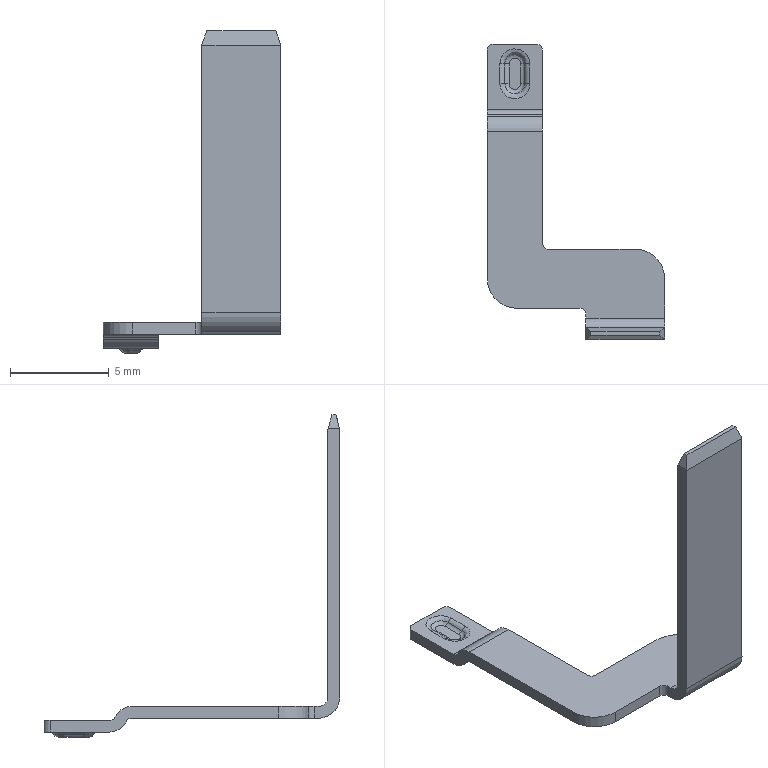Part | STEP file | TQ-DD-1105-THSensorTerminalB1010_デフォルト | 1 solid | 50 faces | box 9 x 15 x 16.36 mm | volume 71.439 mm3 | plane 22 | cylinder 20 | spline 8 | commonest cylinder face diameters 0.6 x10 0.52 x4 1.8 x2 3 x2 1 x1 2.2 x1